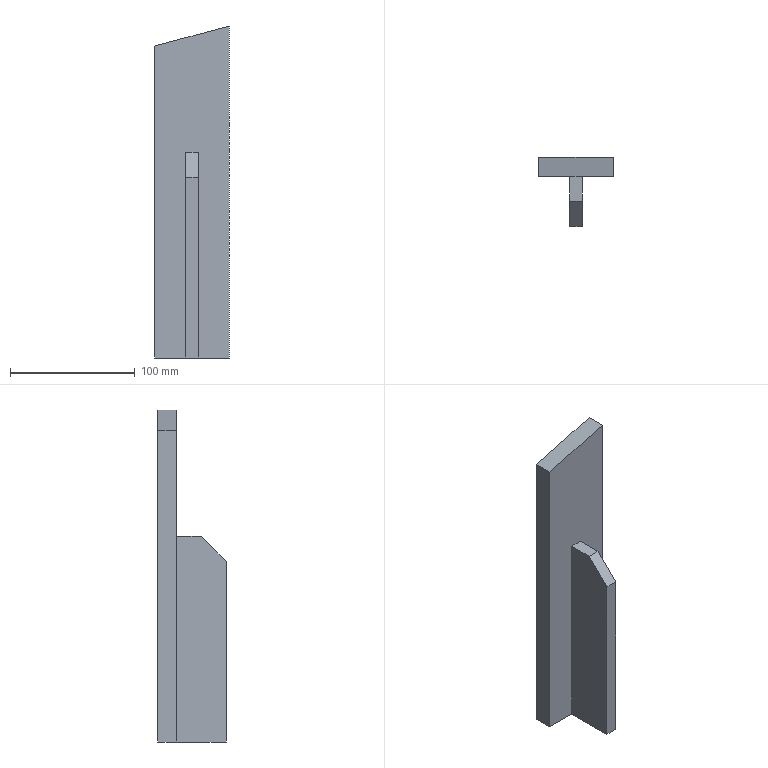Part | NX | features solid 2 | 1 solid | 11 faces | box 60 x 55 x 266.408 mm | volume 296533 mm3 | plane 11
STEP:
#1=CARTESIAN_POINT('',(735.,877.5,-290.));
#2=VERTEX_POINT('',#1);
#3=CARTESIAN_POINT('',(675.,877.5,-290.));
#4=VERTEX_POINT('',#3);
#5=CARTESIAN_POINT('',(735.,877.5,-290.));
#6=DIRECTION('',(-1.,0.,0.));
#7=VECTOR('',#6,1000.);
#8=LINE('',#5,#7);
#9=EDGE_CURVE('',#2,#4,#8,.T.);
#10=ORIENTED_EDGE('',*,*,#9,.F.);
#11=CARTESIAN_POINT('',(735.,862.5,-290.));
#12=VERTEX_POINT('',#11);
#13=CARTESIAN_POINT('',(735.,877.5,-290.));
#14=DIRECTION('',(0.,1.,0.));
#15=VECTOR('',#14,1000.);
#16=LINE('',#13,#15);
#17=EDGE_CURVE('',#12,#2,#16,.T.);
#18=ORIENTED_EDGE('',*,*,#17,.F.);
#19=CARTESIAN_POINT('',(710.,862.5,-290.));
#20=VERTEX_POINT('',#19);
#21=CARTESIAN_POINT('',(735.,862.5,-290.));
#22=DIRECTION('',(-1.,0.,0.));
#23=VECTOR('',#22,1000.);
#24=LINE('',#21,#23);
#25=EDGE_CURVE('',#12,#20,#24,.T.);
#26=ORIENTED_EDGE('',*,*,#25,.T.);
#27=CARTESIAN_POINT('',(710.,822.5,-290.));
#28=VERTEX_POINT('',#27);
#29=CARTESIAN_POINT('',(710.,862.5,-290.));
#30=DIRECTION('',(0.,-1.,0.));
#31=VECTOR('',#30,1000.);
#32=LINE('',#29,#31);
#33=EDGE_CURVE('',#20,#28,#32,.T.);
#34=ORIENTED_EDGE('',*,*,#33,.T.);
#35=CARTESIAN_POINT('',(700.,822.5,-290.));
#36=VERTEX_POINT('',#35);
#37=CARTESIAN_POINT('',(735.,822.5,-290.));
#38=DIRECTION('',(-1.,0.,0.));
#39=VECTOR('',#38,1000.);
#40=LINE('',#37,#39);
#41=EDGE_CURVE('',#28,#36,#40,.T.);
#42=ORIENTED_EDGE('',*,*,#41,.T.);
#43=CARTESIAN_POINT('',(700.,862.5,-290.));
#44=VERTEX_POINT('',#43);
#45=CARTESIAN_POINT('',(700.,862.5,-290.));
#46=DIRECTION('',(0.,-1.,0.));
#47=VECTOR('',#46,1000.);
#48=LINE('',#45,#47);
#49=EDGE_CURVE('',#44,#36,#48,.T.);
#50=ORIENTED_EDGE('',*,*,#49,.F.);
#51=CARTESIAN_POINT('',(675.,862.5,-290.));
#52=VERTEX_POINT('',#51);
#53=CARTESIAN_POINT('',(735.,862.5,-290.));
#54=DIRECTION('',(-1.,0.,0.));
#55=VECTOR('',#54,1000.);
#56=LINE('',#53,#55);
#57=EDGE_CURVE('',#44,#52,#56,.T.);
#58=ORIENTED_EDGE('',*,*,#57,.T.);
#59=CARTESIAN_POINT('',(675.,870.,-290.));
#60=DIRECTION('',(0.,-1.,0.));
#61=VECTOR('',#60,1000.);
#62=LINE('',#59,#61);
#63=EDGE_CURVE('',#52,#4,#62,.F.);
#64=ORIENTED_EDGE('',*,*,#63,.T.);
#65=EDGE_LOOP('',(#10,#18,#26,#34,#42,#50,#58,#64));
#66=FACE_BOUND('',#65,.T.);
#67=CARTESIAN_POINT('',(735.,877.5,-290.));
#68=DIRECTION('',(0.,0.,-1.));
#69=DIRECTION('',(1.,0.,0.));
#70=AXIS2_PLACEMENT_3D('',#67,#68,#69);
#71=PLANE('',#70);
#72=ADVANCED_FACE('',(#66),#71,.T.);
#73=CARTESIAN_POINT('',(710.,842.5,-125.));
#74=VERTEX_POINT('',#73);
#75=CARTESIAN_POINT('',(710.,822.5,-145.));
#76=VERTEX_POINT('',#75);
#77=CARTESIAN_POINT('',(710.,822.5,-145.));
#78=DIRECTION('',(0.,-0.7071,-0.7071));
#79=VECTOR('',#78,1000.);
#80=LINE('',#77,#79);
#81=EDGE_CURVE('',#74,#76,#80,.T.);
#82=ORIENTED_EDGE('',*,*,#81,.F.);
#83=CARTESIAN_POINT('',(700.,842.5,-125.));
#84=VERTEX_POINT('',#83);
#85=CARTESIAN_POINT('',(705.,842.5,-125.));
#86=DIRECTION('',(-1.,0.,0.));
#87=VECTOR('',#86,1000.);
#88=LINE('',#85,#87);
#89=EDGE_CURVE('',#84,#74,#88,.F.);
#90=ORIENTED_EDGE('',*,*,#89,.F.);
#91=CARTESIAN_POINT('',(700.,822.5,-145.));
#92=VERTEX_POINT('',#91);
#93=CARTESIAN_POINT('',(700.,752.5,-215.));
#94=DIRECTION('',(0.,0.7071,0.7071));
#95=VECTOR('',#94,1000.);
#96=LINE('',#93,#95);
#97=EDGE_CURVE('',#92,#84,#96,.T.);
#98=ORIENTED_EDGE('',*,*,#97,.F.);
#99=CARTESIAN_POINT('',(705.,822.5,-145.));
#100=DIRECTION('',(-1.,0.,0.));
#101=VECTOR('',#100,1000.);
#102=LINE('',#99,#101);
#103=EDGE_CURVE('',#76,#92,#102,.T.);
#104=ORIENTED_EDGE('',*,*,#103,.F.);
#105=EDGE_LOOP('',(#82,#90,#98,#104));
#106=FACE_BOUND('',#105,.T.);
#107=CARTESIAN_POINT('',(705.,822.5,-145.));
#108=DIRECTION('',(0.,-0.7071,0.7071));
#109=DIRECTION('',(0.,0.7071,0.7071));
#110=AXIS2_PLACEMENT_3D('',#107,#108,#109);
#111=PLANE('',#110);
#112=ADVANCED_FACE('',(#106),#111,.T.);
#113=CARTESIAN_POINT('',(700.,862.5,-125.));
#114=VERTEX_POINT('',#113);
#115=CARTESIAN_POINT('',(700.,862.5,-125.));
#116=DIRECTION('',(0.,-1.,0.));
#117=VECTOR('',#116,1000.);
#118=LINE('',#115,#117);
#119=EDGE_CURVE('',#114,#84,#118,.T.);
#120=ORIENTED_EDGE('',*,*,#119,.T.);
#121=ORIENTED_EDGE('',*,*,#89,.T.);
#122=CARTESIAN_POINT('',(710.,862.5,-125.));
#123=VERTEX_POINT('',#122);
#124=CARTESIAN_POINT('',(710.,862.5,-125.));
#125=DIRECTION('',(0.,-1.,0.));
#126=VECTOR('',#125,1000.);
#127=LINE('',#124,#126);
#128=EDGE_CURVE('',#123,#74,#127,.T.);
#129=ORIENTED_EDGE('',*,*,#128,.F.);
#130=CARTESIAN_POINT('',(705.,862.5,-125.));
#131=DIRECTION('',(-1.,0.,0.));
#132=VECTOR('',#131,1000.);
#133=LINE('',#130,#132);
#134=EDGE_CURVE('',#123,#114,#133,.T.);
#135=ORIENTED_EDGE('',*,*,#134,.T.);
#136=EDGE_LOOP('',(#120,#121,#129,#135));
#137=FACE_BOUND('',#136,.T.);
#138=CARTESIAN_POINT('',(705.,862.5,-125.));
#139=DIRECTION('',(0.,0.,-1.));
#140=DIRECTION('',(0.,-1.,0.));
#141=AXIS2_PLACEMENT_3D('',#138,#139,#140);
#142=PLANE('',#141);
#143=ADVANCED_FACE('',(#137),#142,.F.);
#144=CARTESIAN_POINT('',(735.,862.5,-23.592));
#145=VERTEX_POINT('',#144);
#146=CARTESIAN_POINT('',(675.,862.5,-39.669));
#147=VERTEX_POINT('',#146);
#148=CARTESIAN_POINT('',(727.913,862.5,-25.491));
#149=DIRECTION('',(-0.9659,0.,-0.2588));
#150=VECTOR('',#149,1000.);
#151=LINE('',#148,#150);
#152=EDGE_CURVE('',#145,#147,#151,.T.);
#153=ORIENTED_EDGE('',*,*,#152,.T.);
#154=CARTESIAN_POINT('',(675.,862.5,-66.379));
#155=DIRECTION('',(0.,0.,1.));
#156=VECTOR('',#155,1000.);
#157=LINE('',#154,#156);
#158=EDGE_CURVE('',#147,#52,#157,.F.);
#159=ORIENTED_EDGE('',*,*,#158,.T.);
#160=ORIENTED_EDGE('',*,*,#57,.F.);
#161=CARTESIAN_POINT('',(700.,862.5,-325.));
#162=DIRECTION('',(0.,0.,1.));
#163=VECTOR('',#162,1000.);
#164=LINE('',#161,#163);
#165=EDGE_CURVE('',#44,#114,#164,.T.);
#166=ORIENTED_EDGE('',*,*,#165,.T.);
#167=ORIENTED_EDGE('',*,*,#134,.F.);
#168=CARTESIAN_POINT('',(710.,862.5,-325.));
#169=DIRECTION('',(0.,0.,1.));
#170=VECTOR('',#169,1000.);
#171=LINE('',#168,#170);
#172=EDGE_CURVE('',#20,#123,#171,.T.);
#173=ORIENTED_EDGE('',*,*,#172,.F.);
#174=ORIENTED_EDGE('',*,*,#25,.F.);
#175=CARTESIAN_POINT('',(735.,862.5,-36.795));
#176=DIRECTION('',(0.,0.,-1.));
#177=VECTOR('',#176,1000.);
#178=LINE('',#175,#177);
#179=EDGE_CURVE('',#145,#12,#178,.T.);
#180=ORIENTED_EDGE('',*,*,#179,.F.);
#181=EDGE_LOOP('',(#153,#159,#160,#166,#167,#173,#174,#180));
#182=FACE_BOUND('',#181,.T.);
#183=CARTESIAN_POINT('',(730.942,862.5,-36.795));
#184=DIRECTION('',(0.,-1.,0.));
#185=DIRECTION('',(1.,0.,0.));
#186=AXIS2_PLACEMENT_3D('',#183,#184,#185);
#187=PLANE('',#186);
#188=ADVANCED_FACE('',(#182),#187,.T.);
#189=CARTESIAN_POINT('',(700.,822.5,-325.));
#190=DIRECTION('',(0.,0.,1.));
#191=VECTOR('',#190,1000.);
#192=LINE('',#189,#191);
#193=EDGE_CURVE('',#36,#92,#192,.T.);
#194=ORIENTED_EDGE('',*,*,#193,.T.);
#195=ORIENTED_EDGE('',*,*,#97,.T.);
#196=ORIENTED_EDGE('',*,*,#119,.F.);
#197=ORIENTED_EDGE('',*,*,#165,.F.);
#198=ORIENTED_EDGE('',*,*,#49,.T.);
#199=EDGE_LOOP('',(#194,#195,#196,#197,#198));
#200=FACE_BOUND('',#199,.T.);
#201=CARTESIAN_POINT('',(700.,862.5,-325.));
#202=DIRECTION('',(-1.,0.,0.));
#203=DIRECTION('',(0.,-1.,0.));
#204=AXIS2_PLACEMENT_3D('',#201,#202,#203);
#205=PLANE('',#204);
#206=ADVANCED_FACE('',(#200),#205,.T.);
#207=CARTESIAN_POINT('',(710.,822.5,-325.));
#208=DIRECTION('',(0.,0.,1.));
#209=VECTOR('',#208,1000.);
#210=LINE('',#207,#209);
#211=EDGE_CURVE('',#28,#76,#210,.T.);
#212=ORIENTED_EDGE('',*,*,#211,.T.);
#213=ORIENTED_EDGE('',*,*,#103,.T.);
#214=ORIENTED_EDGE('',*,*,#193,.F.);
#215=ORIENTED_EDGE('',*,*,#41,.F.);
#216=EDGE_LOOP('',(#212,#213,#214,#215));
#217=FACE_BOUND('',#216,.T.);
#218=CARTESIAN_POINT('',(705.,822.5,-325.));
#219=DIRECTION('',(0.,-1.,0.));
#220=DIRECTION('',(0.,0.,1.));
#221=AXIS2_PLACEMENT_3D('',#218,#219,#220);
#222=PLANE('',#221);
#223=ADVANCED_FACE('',(#217),#222,.T.);
#224=ORIENTED_EDGE('',*,*,#128,.T.);
#225=ORIENTED_EDGE('',*,*,#81,.T.);
#226=ORIENTED_EDGE('',*,*,#211,.F.);
#227=ORIENTED_EDGE('',*,*,#33,.F.);
#228=ORIENTED_EDGE('',*,*,#172,.T.);
#229=EDGE_LOOP('',(#224,#225,#226,#227,#228));
#230=FACE_BOUND('',#229,.T.);
#231=CARTESIAN_POINT('',(710.,862.5,-325.));
#232=DIRECTION('',(-1.,0.,0.));
#233=DIRECTION('',(0.,-1.,0.));
#234=AXIS2_PLACEMENT_3D('',#231,#232,#233);
#235=PLANE('',#234);
#236=ADVANCED_FACE('',(#230),#235,.F.);
#237=ORIENTED_EDGE('',*,*,#179,.T.);
#238=ORIENTED_EDGE('',*,*,#17,.T.);
#239=CARTESIAN_POINT('',(735.,877.5,-23.592));
#240=VERTEX_POINT('',#239);
#241=CARTESIAN_POINT('',(735.,877.5,-36.795));
#242=DIRECTION('',(0.,0.,-1.));
#243=VECTOR('',#242,1000.);
#244=LINE('',#241,#243);
#245=EDGE_CURVE('',#240,#2,#244,.T.);
#246=ORIENTED_EDGE('',*,*,#245,.F.);
#247=CARTESIAN_POINT('',(735.,870.,-23.592));
#248=DIRECTION('',(0.,1.,0.));
#249=VECTOR('',#248,1000.);
#250=LINE('',#247,#249);
#251=EDGE_CURVE('',#145,#240,#250,.T.);
#252=ORIENTED_EDGE('',*,*,#251,.F.);
#253=EDGE_LOOP('',(#237,#238,#246,#252));
#254=FACE_BOUND('',#253,.T.);
#255=CARTESIAN_POINT('',(735.,870.,-36.795));
#256=DIRECTION('',(-1.,0.,0.));
#257=DIRECTION('',(0.,0.,-1.));
#258=AXIS2_PLACEMENT_3D('',#255,#256,#257);
#259=PLANE('',#258);
#260=ADVANCED_FACE('',(#254),#259,.F.);
#261=ORIENTED_EDGE('',*,*,#245,.T.);
#262=ORIENTED_EDGE('',*,*,#9,.T.);
#263=CARTESIAN_POINT('',(675.,877.5,-39.669));
#264=VERTEX_POINT('',#263);
#265=CARTESIAN_POINT('',(675.,877.5,-66.379));
#266=DIRECTION('',(0.,0.,1.));
#267=VECTOR('',#266,1000.);
#268=LINE('',#265,#267);
#269=EDGE_CURVE('',#264,#4,#268,.F.);
#270=ORIENTED_EDGE('',*,*,#269,.F.);
#271=CARTESIAN_POINT('',(727.913,877.5,-25.491));
#272=DIRECTION('',(-0.9659,0.,-0.2588));
#273=VECTOR('',#272,1000.);
#274=LINE('',#271,#273);
#275=EDGE_CURVE('',#240,#264,#274,.T.);
#276=ORIENTED_EDGE('',*,*,#275,.F.);
#277=EDGE_LOOP('',(#261,#262,#270,#276));
#278=FACE_BOUND('',#277,.T.);
#279=CARTESIAN_POINT('',(730.942,877.5,-36.795));
#280=DIRECTION('',(0.,-1.,0.));
#281=DIRECTION('',(1.,0.,0.));
#282=AXIS2_PLACEMENT_3D('',#279,#280,#281);
#283=PLANE('',#282);
#284=ADVANCED_FACE('',(#278),#283,.F.);
#285=ORIENTED_EDGE('',*,*,#269,.T.);
#286=ORIENTED_EDGE('',*,*,#63,.F.);
#287=ORIENTED_EDGE('',*,*,#158,.F.);
#288=CARTESIAN_POINT('',(675.,870.,-39.669));
#289=DIRECTION('',(0.,1.,0.));
#290=VECTOR('',#289,1000.);
#291=LINE('',#288,#290);
#292=EDGE_CURVE('',#264,#147,#291,.F.);
#293=ORIENTED_EDGE('',*,*,#292,.F.);
#294=EDGE_LOOP('',(#285,#286,#287,#293));
#295=FACE_BOUND('',#294,.T.);
#296=CARTESIAN_POINT('',(675.,870.,-66.379));
#297=DIRECTION('',(-1.,0.,0.));
#298=DIRECTION('',(0.,0.,-1.));
#299=AXIS2_PLACEMENT_3D('',#296,#297,#298);
#300=PLANE('',#299);
#301=ADVANCED_FACE('',(#295),#300,.T.);
#302=ORIENTED_EDGE('',*,*,#152,.F.);
#303=ORIENTED_EDGE('',*,*,#251,.T.);
#304=ORIENTED_EDGE('',*,*,#275,.T.);
#305=ORIENTED_EDGE('',*,*,#292,.T.);
#306=EDGE_LOOP('',(#302,#303,#304,#305));
#307=FACE_BOUND('',#306,.T.);
#308=CARTESIAN_POINT('',(693.409,920.,-34.736));
#309=DIRECTION('',(0.2588,0.,-0.9659));
#310=DIRECTION('',(0.9659,0.,0.2588));
#311=AXIS2_PLACEMENT_3D('',#308,#309,#310);
#312=PLANE('',#311);
#313=ADVANCED_FACE('',(#307),#312,.F.);
#314=CLOSED_SHELL('',(#72,#112,#143,#188,#206,#223,#236,#260,#284,#301,#313));
#315=MANIFOLD_SOLID_BREP('',#314);
#316=(LENGTH_UNIT()NAMED_UNIT(*)SI_UNIT(.MILLI.,.METRE.));
#317=UNCERTAINTY_MEASURE_WITH_UNIT(LENGTH_MEASURE(0.00001),#316,'','');
#318=(NAMED_UNIT(*)PLANE_ANGLE_UNIT()SI_UNIT($,.RADIAN.));
#319=(NAMED_UNIT(*)SI_UNIT($,.STERADIAN.)SOLID_ANGLE_UNIT());
#320=(GEOMETRIC_REPRESENTATION_CONTEXT(3)GLOBAL_UNCERTAINTY_ASSIGNED_CONTEXT((#317))GLOBAL_UNIT_ASSIGNED_CONTEXT((#316,#318,#319))REPRESENTATION_CONTEXT('',''));
#321=ADVANCED_BREP_SHAPE_REPRESENTATION('',(#315),#320);